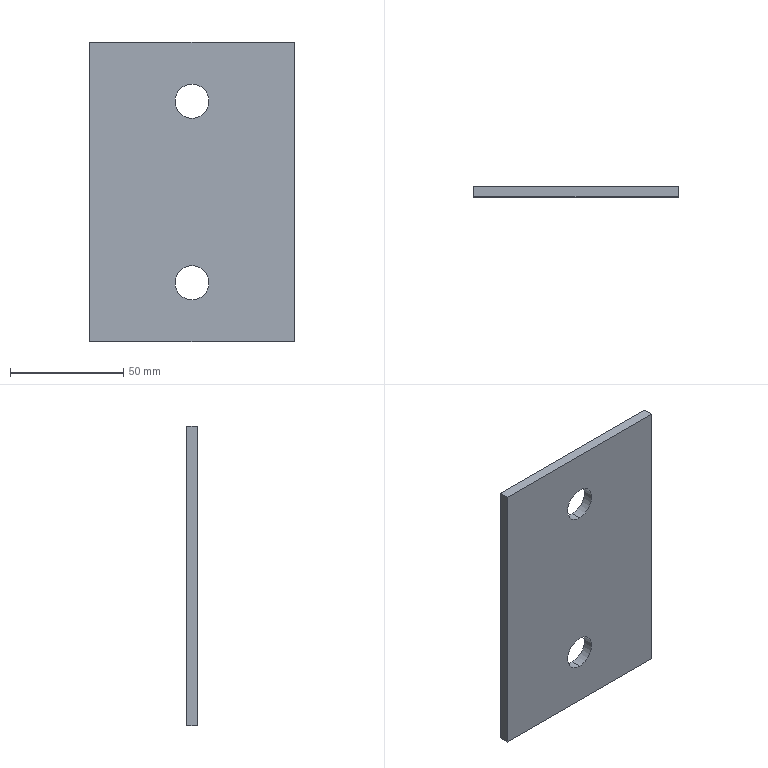Part | SolidWorks | features FlatPattern 1, SMBaseFlange 1, SheetMetal 1 | 1 solid | 10 faces | box 90 x 4.5 x 132 mm | volume 51870 mm3 | plane 6 | cylinder 4 | commonest cylinder face diameters 15 x4
STEP:
#1=CARTESIAN_POINT('',(45.,-4.5,98.5));
#2=VERTEX_POINT('',#1);
#3=CARTESIAN_POINT('',(45.,-4.5,113.5));
#4=VERTEX_POINT('',#3);
#5=CARTESIAN_POINT('',(45.,-4.5,106.));
#6=DIRECTION('',(0.,1.,0.));
#7=DIRECTION('',(0.,0.,1.));
#8=AXIS2_PLACEMENT_3D('',#5,#6,#7);
#9=CIRCLE('',#8,7.5);
#10=EDGE_CURVE('',#2,#4,#9,.T.);
#11=ORIENTED_EDGE('',*,*,#10,.F.);
#12=CARTESIAN_POINT('',(45.,0.,98.5));
#13=VERTEX_POINT('',#12);
#14=CARTESIAN_POINT('',(45.,-4.5,98.5));
#15=DIRECTION('',(0.,1.,0.));
#16=VECTOR('',#15,1000.);
#17=LINE('',#14,#16);
#18=EDGE_CURVE('',#2,#13,#17,.T.);
#19=ORIENTED_EDGE('',*,*,#18,.T.);
#20=CARTESIAN_POINT('',(45.,0.,113.5));
#21=VERTEX_POINT('',#20);
#22=CARTESIAN_POINT('',(45.,0.,106.));
#23=DIRECTION('',(0.,1.,0.));
#24=DIRECTION('',(0.,0.,1.));
#25=AXIS2_PLACEMENT_3D('',#22,#23,#24);
#26=CIRCLE('',#25,7.5);
#27=EDGE_CURVE('',#13,#21,#26,.T.);
#28=ORIENTED_EDGE('',*,*,#27,.T.);
#29=CARTESIAN_POINT('',(45.,-4.5,113.5));
#30=DIRECTION('',(0.,1.,0.));
#31=VECTOR('',#30,1000.);
#32=LINE('',#29,#31);
#33=EDGE_CURVE('',#4,#21,#32,.T.);
#34=ORIENTED_EDGE('',*,*,#33,.F.);
#35=EDGE_LOOP('',(#11,#19,#28,#34));
#36=FACE_OUTER_BOUND('',#35,.T.);
#37=CARTESIAN_POINT('',(45.,-4.5,106.));
#38=DIRECTION('',(0.,1.,0.));
#39=DIRECTION('',(0.,0.,1.));
#40=AXIS2_PLACEMENT_3D('',#37,#38,#39);
#41=CYLINDRICAL_SURFACE('',#40,7.5);
#42=ADVANCED_FACE('',(#36),#41,.F.);
#43=CARTESIAN_POINT('',(45.,-4.5,18.5));
#44=VERTEX_POINT('',#43);
#45=CARTESIAN_POINT('',(45.,-4.5,33.5));
#46=VERTEX_POINT('',#45);
#47=CARTESIAN_POINT('',(45.,-4.5,26.));
#48=DIRECTION('',(0.,1.,0.));
#49=DIRECTION('',(0.,0.,1.));
#50=AXIS2_PLACEMENT_3D('',#47,#48,#49);
#51=CIRCLE('',#50,7.5);
#52=EDGE_CURVE('',#44,#46,#51,.T.);
#53=ORIENTED_EDGE('',*,*,#52,.F.);
#54=CARTESIAN_POINT('',(45.,0.,18.5));
#55=VERTEX_POINT('',#54);
#56=CARTESIAN_POINT('',(45.,-4.5,18.5));
#57=DIRECTION('',(0.,1.,0.));
#58=VECTOR('',#57,1000.);
#59=LINE('',#56,#58);
#60=EDGE_CURVE('',#44,#55,#59,.T.);
#61=ORIENTED_EDGE('',*,*,#60,.T.);
#62=CARTESIAN_POINT('',(45.,0.,33.5));
#63=VERTEX_POINT('',#62);
#64=CARTESIAN_POINT('',(45.,0.,26.));
#65=DIRECTION('',(0.,1.,0.));
#66=DIRECTION('',(0.,0.,1.));
#67=AXIS2_PLACEMENT_3D('',#64,#65,#66);
#68=CIRCLE('',#67,7.5);
#69=EDGE_CURVE('',#55,#63,#68,.T.);
#70=ORIENTED_EDGE('',*,*,#69,.T.);
#71=CARTESIAN_POINT('',(45.,-4.5,33.5));
#72=DIRECTION('',(0.,1.,0.));
#73=VECTOR('',#72,1000.);
#74=LINE('',#71,#73);
#75=EDGE_CURVE('',#46,#63,#74,.T.);
#76=ORIENTED_EDGE('',*,*,#75,.F.);
#77=EDGE_LOOP('',(#53,#61,#70,#76));
#78=FACE_OUTER_BOUND('',#77,.T.);
#79=CARTESIAN_POINT('',(45.,-4.5,26.));
#80=DIRECTION('',(0.,1.,0.));
#81=DIRECTION('',(0.,0.,1.));
#82=AXIS2_PLACEMENT_3D('',#79,#80,#81);
#83=CYLINDRICAL_SURFACE('',#82,7.5);
#84=ADVANCED_FACE('',(#78),#83,.F.);
#85=CARTESIAN_POINT('',(0.,0.,0.));
#86=VERTEX_POINT('',#85);
#87=CARTESIAN_POINT('',(0.,0.,132.));
#88=VERTEX_POINT('',#87);
#89=CARTESIAN_POINT('',(0.,0.,0.));
#90=DIRECTION('',(0.,0.,1.));
#91=VECTOR('',#90,1000.);
#92=LINE('',#89,#91);
#93=EDGE_CURVE('',#86,#88,#92,.T.);
#94=ORIENTED_EDGE('',*,*,#93,.F.);
#95=CARTESIAN_POINT('',(0.,-4.5,0.));
#96=VERTEX_POINT('',#95);
#97=CARTESIAN_POINT('',(0.,-4.5,0.));
#98=DIRECTION('',(0.,1.,0.));
#99=VECTOR('',#98,1000.);
#100=LINE('',#97,#99);
#101=EDGE_CURVE('',#96,#86,#100,.T.);
#102=ORIENTED_EDGE('',*,*,#101,.F.);
#103=CARTESIAN_POINT('',(0.,-4.5,132.));
#104=VERTEX_POINT('',#103);
#105=CARTESIAN_POINT('',(0.,-4.5,0.));
#106=DIRECTION('',(0.,0.,1.));
#107=VECTOR('',#106,1000.);
#108=LINE('',#105,#107);
#109=EDGE_CURVE('',#96,#104,#108,.T.);
#110=ORIENTED_EDGE('',*,*,#109,.T.);
#111=CARTESIAN_POINT('',(0.,-4.5,132.));
#112=DIRECTION('',(0.,1.,0.));
#113=VECTOR('',#112,1000.);
#114=LINE('',#111,#113);
#115=EDGE_CURVE('',#104,#88,#114,.T.);
#116=ORIENTED_EDGE('',*,*,#115,.T.);
#117=EDGE_LOOP('',(#94,#102,#110,#116));
#118=FACE_OUTER_BOUND('',#117,.T.);
#119=CARTESIAN_POINT('',(0.,-4.5,0.));
#120=DIRECTION('',(-1.,0.,0.));
#121=DIRECTION('',(0.,0.,1.));
#122=AXIS2_PLACEMENT_3D('',#119,#120,#121);
#123=PLANE('',#122);
#124=ADVANCED_FACE('',(#118),#123,.T.);
#125=CARTESIAN_POINT('',(90.,0.,0.));
#126=VERTEX_POINT('',#125);
#127=CARTESIAN_POINT('',(0.,0.,0.));
#128=DIRECTION('',(-1.,0.,0.));
#129=VECTOR('',#128,1000.);
#130=LINE('',#127,#129);
#131=EDGE_CURVE('',#126,#86,#130,.T.);
#132=ORIENTED_EDGE('',*,*,#131,.F.);
#133=CARTESIAN_POINT('',(90.,-4.5,0.));
#134=VERTEX_POINT('',#133);
#135=CARTESIAN_POINT('',(90.,-4.5,0.));
#136=DIRECTION('',(0.,1.,0.));
#137=VECTOR('',#136,1000.);
#138=LINE('',#135,#137);
#139=EDGE_CURVE('',#134,#126,#138,.T.);
#140=ORIENTED_EDGE('',*,*,#139,.F.);
#141=CARTESIAN_POINT('',(0.,-4.5,0.));
#142=DIRECTION('',(-1.,0.,0.));
#143=VECTOR('',#142,1000.);
#144=LINE('',#141,#143);
#145=EDGE_CURVE('',#134,#96,#144,.T.);
#146=ORIENTED_EDGE('',*,*,#145,.T.);
#147=ORIENTED_EDGE('',*,*,#101,.T.);
#148=EDGE_LOOP('',(#132,#140,#146,#147));
#149=FACE_OUTER_BOUND('',#148,.T.);
#150=CARTESIAN_POINT('',(0.,-4.5,0.));
#151=DIRECTION('',(0.,0.,-1.));
#152=DIRECTION('',(-1.,0.,0.));
#153=AXIS2_PLACEMENT_3D('',#150,#151,#152);
#154=PLANE('',#153);
#155=ADVANCED_FACE('',(#149),#154,.T.);
#156=CARTESIAN_POINT('',(90.,0.,132.));
#157=VERTEX_POINT('',#156);
#158=CARTESIAN_POINT('',(90.,0.,0.));
#159=DIRECTION('',(0.,0.,-1.));
#160=VECTOR('',#159,1000.);
#161=LINE('',#158,#160);
#162=EDGE_CURVE('',#157,#126,#161,.T.);
#163=ORIENTED_EDGE('',*,*,#162,.F.);
#164=CARTESIAN_POINT('',(90.,-4.5,132.));
#165=VERTEX_POINT('',#164);
#166=CARTESIAN_POINT('',(90.,-4.5,132.));
#167=DIRECTION('',(0.,1.,0.));
#168=VECTOR('',#167,1000.);
#169=LINE('',#166,#168);
#170=EDGE_CURVE('',#165,#157,#169,.T.);
#171=ORIENTED_EDGE('',*,*,#170,.F.);
#172=CARTESIAN_POINT('',(90.,-4.5,0.));
#173=DIRECTION('',(0.,0.,-1.));
#174=VECTOR('',#173,1000.);
#175=LINE('',#172,#174);
#176=EDGE_CURVE('',#165,#134,#175,.T.);
#177=ORIENTED_EDGE('',*,*,#176,.T.);
#178=ORIENTED_EDGE('',*,*,#139,.T.);
#179=EDGE_LOOP('',(#163,#171,#177,#178));
#180=FACE_OUTER_BOUND('',#179,.T.);
#181=CARTESIAN_POINT('',(90.,-4.5,0.));
#182=DIRECTION('',(1.,0.,0.));
#183=DIRECTION('',(0.,0.,-1.));
#184=AXIS2_PLACEMENT_3D('',#181,#182,#183);
#185=PLANE('',#184);
#186=ADVANCED_FACE('',(#180),#185,.T.);
#187=CARTESIAN_POINT('',(0.,0.,132.));
#188=DIRECTION('',(1.,0.,0.));
#189=VECTOR('',#188,1000.);
#190=LINE('',#187,#189);
#191=EDGE_CURVE('',#88,#157,#190,.T.);
#192=ORIENTED_EDGE('',*,*,#191,.F.);
#193=ORIENTED_EDGE('',*,*,#115,.F.);
#194=CARTESIAN_POINT('',(0.,-4.5,132.));
#195=DIRECTION('',(1.,0.,0.));
#196=VECTOR('',#195,1000.);
#197=LINE('',#194,#196);
#198=EDGE_CURVE('',#104,#165,#197,.T.);
#199=ORIENTED_EDGE('',*,*,#198,.T.);
#200=ORIENTED_EDGE('',*,*,#170,.T.);
#201=EDGE_LOOP('',(#192,#193,#199,#200));
#202=FACE_OUTER_BOUND('',#201,.T.);
#203=CARTESIAN_POINT('',(0.,-4.5,132.));
#204=DIRECTION('',(0.,0.,1.));
#205=DIRECTION('',(1.,0.,0.));
#206=AXIS2_PLACEMENT_3D('',#203,#204,#205);
#207=PLANE('',#206);
#208=ADVANCED_FACE('',(#202),#207,.T.);
#209=CARTESIAN_POINT('',(45.,-4.5,106.));
#210=DIRECTION('',(0.,1.,0.));
#211=DIRECTION('',(0.,0.,1.));
#212=AXIS2_PLACEMENT_3D('',#209,#210,#211);
#213=CIRCLE('',#212,7.5);
#214=EDGE_CURVE('',#4,#2,#213,.T.);
#215=ORIENTED_EDGE('',*,*,#214,.T.);
#216=ORIENTED_EDGE('',*,*,#10,.T.);
#217=EDGE_LOOP('',(#215,#216));
#218=FACE_BOUND('',#217,.T.);
#219=CARTESIAN_POINT('',(45.,-4.5,26.));
#220=DIRECTION('',(0.,1.,0.));
#221=DIRECTION('',(0.,0.,1.));
#222=AXIS2_PLACEMENT_3D('',#219,#220,#221);
#223=CIRCLE('',#222,7.5);
#224=EDGE_CURVE('',#46,#44,#223,.T.);
#225=ORIENTED_EDGE('',*,*,#224,.T.);
#226=ORIENTED_EDGE('',*,*,#52,.T.);
#227=EDGE_LOOP('',(#225,#226));
#228=FACE_BOUND('',#227,.T.);
#229=ORIENTED_EDGE('',*,*,#109,.F.);
#230=ORIENTED_EDGE('',*,*,#145,.F.);
#231=ORIENTED_EDGE('',*,*,#176,.F.);
#232=ORIENTED_EDGE('',*,*,#198,.F.);
#233=EDGE_LOOP('',(#229,#230,#231,#232));
#234=FACE_OUTER_BOUND('',#233,.T.);
#235=CARTESIAN_POINT('',(0.,-4.5,0.));
#236=DIRECTION('',(0.,1.,0.));
#237=DIRECTION('',(0.,0.,1.));
#238=AXIS2_PLACEMENT_3D('',#235,#236,#237);
#239=PLANE('',#238);
#240=ADVANCED_FACE('',(#218,#228,#234),#239,.F.);
#241=CARTESIAN_POINT('',(45.,0.,106.));
#242=DIRECTION('',(0.,1.,0.));
#243=DIRECTION('',(0.,0.,1.));
#244=AXIS2_PLACEMENT_3D('',#241,#242,#243);
#245=CIRCLE('',#244,7.5);
#246=EDGE_CURVE('',#21,#13,#245,.T.);
#247=ORIENTED_EDGE('',*,*,#246,.F.);
#248=ORIENTED_EDGE('',*,*,#27,.F.);
#249=EDGE_LOOP('',(#247,#248));
#250=FACE_BOUND('',#249,.T.);
#251=CARTESIAN_POINT('',(45.,0.,26.));
#252=DIRECTION('',(0.,1.,0.));
#253=DIRECTION('',(0.,0.,1.));
#254=AXIS2_PLACEMENT_3D('',#251,#252,#253);
#255=CIRCLE('',#254,7.5);
#256=EDGE_CURVE('',#63,#55,#255,.T.);
#257=ORIENTED_EDGE('',*,*,#256,.F.);
#258=ORIENTED_EDGE('',*,*,#69,.F.);
#259=EDGE_LOOP('',(#257,#258));
#260=FACE_BOUND('',#259,.T.);
#261=ORIENTED_EDGE('',*,*,#93,.T.);
#262=ORIENTED_EDGE('',*,*,#191,.T.);
#263=ORIENTED_EDGE('',*,*,#162,.T.);
#264=ORIENTED_EDGE('',*,*,#131,.T.);
#265=EDGE_LOOP('',(#261,#262,#263,#264));
#266=FACE_OUTER_BOUND('',#265,.T.);
#267=CARTESIAN_POINT('',(0.,0.,0.));
#268=DIRECTION('',(0.,1.,0.));
#269=DIRECTION('',(0.,0.,1.));
#270=AXIS2_PLACEMENT_3D('',#267,#268,#269);
#271=PLANE('',#270);
#272=ADVANCED_FACE('',(#250,#260,#266),#271,.T.);
#273=ORIENTED_EDGE('',*,*,#60,.F.);
#274=ORIENTED_EDGE('',*,*,#224,.F.);
#275=ORIENTED_EDGE('',*,*,#75,.T.);
#276=ORIENTED_EDGE('',*,*,#256,.T.);
#277=EDGE_LOOP('',(#273,#274,#275,#276));
#278=FACE_OUTER_BOUND('',#277,.T.);
#279=CARTESIAN_POINT('',(45.,-4.5,26.));
#280=DIRECTION('',(0.,1.,0.));
#281=DIRECTION('',(0.,0.,1.));
#282=AXIS2_PLACEMENT_3D('',#279,#280,#281);
#283=CYLINDRICAL_SURFACE('',#282,7.5);
#284=ADVANCED_FACE('',(#278),#283,.F.);
#285=ORIENTED_EDGE('',*,*,#18,.F.);
#286=ORIENTED_EDGE('',*,*,#214,.F.);
#287=ORIENTED_EDGE('',*,*,#33,.T.);
#288=ORIENTED_EDGE('',*,*,#246,.T.);
#289=EDGE_LOOP('',(#285,#286,#287,#288));
#290=FACE_OUTER_BOUND('',#289,.T.);
#291=CARTESIAN_POINT('',(45.,-4.5,106.));
#292=DIRECTION('',(0.,1.,0.));
#293=DIRECTION('',(0.,0.,1.));
#294=AXIS2_PLACEMENT_3D('',#291,#292,#293);
#295=CYLINDRICAL_SURFACE('',#294,7.5);
#296=ADVANCED_FACE('',(#290),#295,.F.);
#297=CLOSED_SHELL('',(#42,#84,#124,#155,#186,#208,#240,#272,#284,#296));
#298=MANIFOLD_SOLID_BREP('',#297);
#299=CARTESIAN_POINT('',(0.,0.,0.));
#300=DIRECTION('',(0.,0.,1.));
#301=DIRECTION('',(1.,0.,0.));
#302=AXIS2_PLACEMENT_3D('',#299,#300,#301);
#303=(LENGTH_UNIT()NAMED_UNIT(*)SI_UNIT(.MILLI.,.METRE.));
#304=UNCERTAINTY_MEASURE_WITH_UNIT(LENGTH_MEASURE(0.00001),#303,'','');
#305=(NAMED_UNIT(*)PLANE_ANGLE_UNIT()SI_UNIT($,.RADIAN.));
#306=(NAMED_UNIT(*)SI_UNIT($,.STERADIAN.)SOLID_ANGLE_UNIT());
#307=(GEOMETRIC_REPRESENTATION_CONTEXT(3)GLOBAL_UNCERTAINTY_ASSIGNED_CONTEXT((#304))GLOBAL_UNIT_ASSIGNED_CONTEXT((#303,#305,#306))REPRESENTATION_CONTEXT('',''));
#308=ADVANCED_BREP_SHAPE_REPRESENTATION('',(#298,#302),#307);